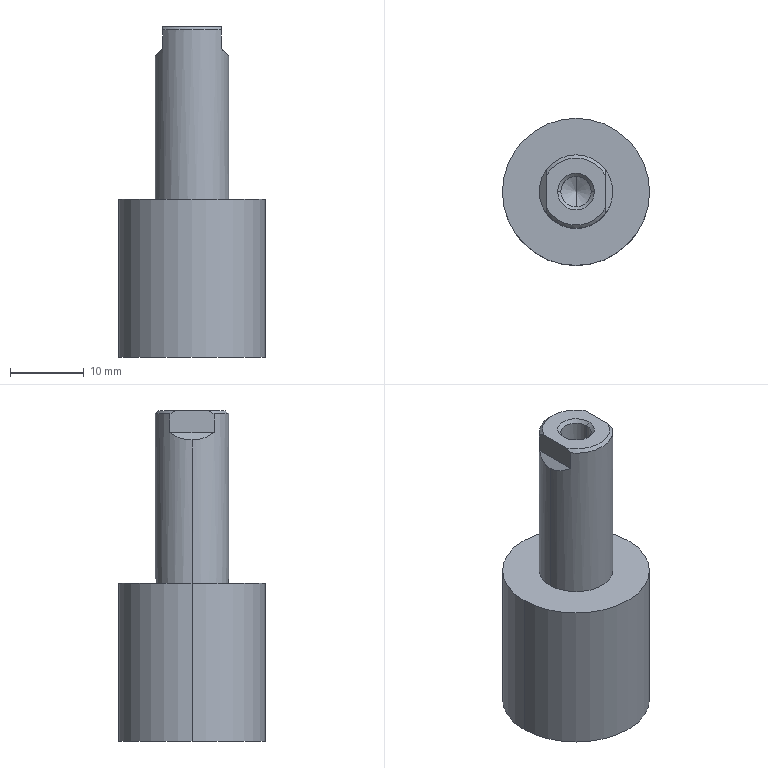Part | STEP file | HI_JSNR20X15_rod_default | 1 solid | 19 faces | box 20 x 20 x 45 mm | volume 8457 mm3 | plane 7 | cylinder 6 | cone 6 | commonest cylinder face diameters 4.134 x2 10 x2 20 x2